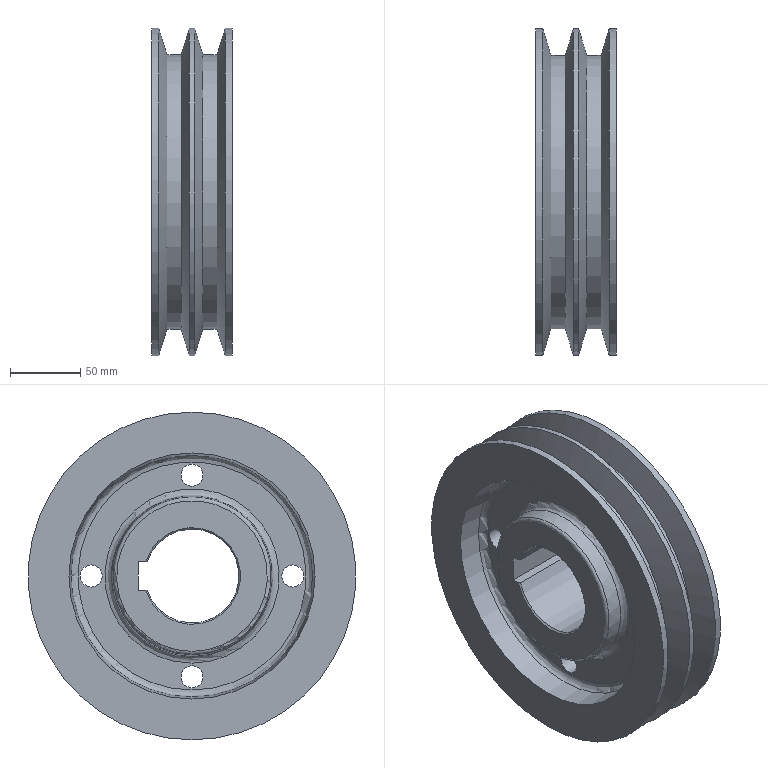Part | NX | features 大带轮_孔板轮(A) 2 | 1 solid | 35 faces | box 57.5 x 233.6 x 233.6 mm | volume 1208197 mm3 | cylinder 10 | cone 10 | plane 9 | torus 6 | commonest cylinder face diameters 15.7 x4 233.6 x3 195.4 x2 67 x1
STEP:
#1=CARTESIAN_POINT('',(21.25,0.,-62.113));
#2=VERTEX_POINT('',#1);
#3=CARTESIAN_POINT('',(21.25,0.,0.));
#4=DIRECTION('',(1.,0.,0.));
#5=DIRECTION('',(0.,0.,-1.));
#6=AXIS2_PLACEMENT_3D('',#3,#4,#5);
#7=CIRCLE('',#6,62.113);
#8=EDGE_CURVE('',#2,#2,#7,.T.);
#9=ORIENTED_EDGE('',*,*,#8,.T.);
#10=EDGE_LOOP('',(#9));
#11=FACE_BOUND('',#10,.T.);
#12=CARTESIAN_POINT('',(21.25,0.,-81.259));
#13=VERTEX_POINT('',#12);
#14=CARTESIAN_POINT('',(21.25,0.,0.));
#15=DIRECTION('',(1.,0.,0.));
#16=DIRECTION('',(0.,0.,-1.));
#17=AXIS2_PLACEMENT_3D('',#14,#15,#16);
#18=CIRCLE('',#17,81.259);
#19=EDGE_CURVE('',#13,#13,#18,.F.);
#20=ORIENTED_EDGE('',*,*,#19,.T.);
#21=EDGE_LOOP('',(#20));
#22=FACE_BOUND('',#21,.T.);
#23=CARTESIAN_POINT('',(21.25,71.85,-7.85));
#24=VERTEX_POINT('',#23);
#25=CARTESIAN_POINT('',(21.25,71.85,0.));
#26=DIRECTION('',(1.,0.,0.));
#27=DIRECTION('',(0.,0.,-1.));
#28=AXIS2_PLACEMENT_3D('',#25,#26,#27);
#29=CIRCLE('',#28,7.85);
#30=EDGE_CURVE('',#24,#24,#29,.F.);
#31=ORIENTED_EDGE('',*,*,#30,.F.);
#32=EDGE_LOOP('',(#31));
#33=FACE_BOUND('',#32,.T.);
#34=CARTESIAN_POINT('',(21.25,0.,-79.7));
#35=VERTEX_POINT('',#34);
#36=CARTESIAN_POINT('',(21.25,0.,-71.85));
#37=DIRECTION('',(1.,0.,0.));
#38=DIRECTION('',(0.,0.,-1.));
#39=AXIS2_PLACEMENT_3D('',#36,#37,#38);
#40=CIRCLE('',#39,7.85);
#41=EDGE_CURVE('',#35,#35,#40,.F.);
#42=ORIENTED_EDGE('',*,*,#41,.F.);
#43=EDGE_LOOP('',(#42));
#44=FACE_BOUND('',#43,.T.);
#45=CARTESIAN_POINT('',(21.25,-71.85,-7.85));
#46=VERTEX_POINT('',#45);
#47=CARTESIAN_POINT('',(21.25,-71.85,0.));
#48=DIRECTION('',(1.,0.,0.));
#49=DIRECTION('',(0.,0.,-1.));
#50=AXIS2_PLACEMENT_3D('',#47,#48,#49);
#51=CIRCLE('',#50,7.85);
#52=EDGE_CURVE('',#46,#46,#51,.F.);
#53=ORIENTED_EDGE('',*,*,#52,.F.);
#54=EDGE_LOOP('',(#53));
#55=FACE_BOUND('',#54,.T.);
#56=CARTESIAN_POINT('',(21.25,0.,64.));
#57=VERTEX_POINT('',#56);
#58=CARTESIAN_POINT('',(21.25,0.,71.85));
#59=DIRECTION('',(1.,0.,0.));
#60=DIRECTION('',(0.,0.,-1.));
#61=AXIS2_PLACEMENT_3D('',#58,#59,#60);
#62=CIRCLE('',#61,7.85);
#63=EDGE_CURVE('',#57,#57,#62,.F.);
#64=ORIENTED_EDGE('',*,*,#63,.F.);
#65=EDGE_LOOP('',(#64));
#66=FACE_BOUND('',#65,.T.);
#67=CARTESIAN_POINT('',(21.25,57.531,0.));
#68=DIRECTION('',(1.,0.,0.));
#69=DIRECTION('',(0.,0.,-1.));
#70=AXIS2_PLACEMENT_3D('',#67,#68,#69);
#71=PLANE('',#70);
#72=ADVANCED_FACE('',(#11,#22,#33,#44,#55,#66),#71,.F.);
#73=CARTESIAN_POINT('',(36.25,0.,62.113));
#74=VERTEX_POINT('',#73);
#75=CARTESIAN_POINT('',(36.25,0.,0.));
#76=DIRECTION('',(-1.,0.,0.));
#77=DIRECTION('',(0.,0.,1.));
#78=AXIS2_PLACEMENT_3D('',#75,#76,#77);
#79=CIRCLE('',#78,62.113);
#80=EDGE_CURVE('',#74,#74,#79,.T.);
#81=ORIENTED_EDGE('',*,*,#80,.T.);
#82=EDGE_LOOP('',(#81));
#83=FACE_BOUND('',#82,.T.);
#84=CARTESIAN_POINT('',(36.25,0.,81.259));
#85=VERTEX_POINT('',#84);
#86=CARTESIAN_POINT('',(36.25,0.,0.));
#87=DIRECTION('',(-1.,0.,0.));
#88=DIRECTION('',(0.,0.,1.));
#89=AXIS2_PLACEMENT_3D('',#86,#87,#88);
#90=CIRCLE('',#89,81.259);
#91=EDGE_CURVE('',#85,#85,#90,.F.);
#92=ORIENTED_EDGE('',*,*,#91,.T.);
#93=EDGE_LOOP('',(#92));
#94=FACE_BOUND('',#93,.T.);
#95=CARTESIAN_POINT('',(36.25,71.85,7.85));
#96=VERTEX_POINT('',#95);
#97=CARTESIAN_POINT('',(36.25,71.85,0.));
#98=DIRECTION('',(-1.,0.,0.));
#99=DIRECTION('',(0.,0.,1.));
#100=AXIS2_PLACEMENT_3D('',#97,#98,#99);
#101=CIRCLE('',#100,7.85);
#102=EDGE_CURVE('',#96,#96,#101,.F.);
#103=ORIENTED_EDGE('',*,*,#102,.F.);
#104=EDGE_LOOP('',(#103));
#105=FACE_BOUND('',#104,.T.);
#106=CARTESIAN_POINT('',(36.25,0.,-64.));
#107=VERTEX_POINT('',#106);
#108=CARTESIAN_POINT('',(36.25,0.,-71.85));
#109=DIRECTION('',(-1.,0.,0.));
#110=DIRECTION('',(0.,0.,1.));
#111=AXIS2_PLACEMENT_3D('',#108,#109,#110);
#112=CIRCLE('',#111,7.85);
#113=EDGE_CURVE('',#107,#107,#112,.F.);
#114=ORIENTED_EDGE('',*,*,#113,.F.);
#115=EDGE_LOOP('',(#114));
#116=FACE_BOUND('',#115,.T.);
#117=CARTESIAN_POINT('',(36.25,-71.85,7.85));
#118=VERTEX_POINT('',#117);
#119=CARTESIAN_POINT('',(36.25,-71.85,0.));
#120=DIRECTION('',(-1.,0.,0.));
#121=DIRECTION('',(0.,0.,1.));
#122=AXIS2_PLACEMENT_3D('',#119,#120,#121);
#123=CIRCLE('',#122,7.85);
#124=EDGE_CURVE('',#118,#118,#123,.F.);
#125=ORIENTED_EDGE('',*,*,#124,.F.);
#126=EDGE_LOOP('',(#125));
#127=FACE_BOUND('',#126,.T.);
#128=CARTESIAN_POINT('',(36.25,0.,79.7));
#129=VERTEX_POINT('',#128);
#130=CARTESIAN_POINT('',(36.25,0.,71.85));
#131=DIRECTION('',(-1.,0.,0.));
#132=DIRECTION('',(0.,0.,1.));
#133=AXIS2_PLACEMENT_3D('',#130,#131,#132);
#134=CIRCLE('',#133,7.85);
#135=EDGE_CURVE('',#129,#129,#134,.F.);
#136=ORIENTED_EDGE('',*,*,#135,.F.);
#137=EDGE_LOOP('',(#136));
#138=FACE_BOUND('',#137,.T.);
#139=CARTESIAN_POINT('',(36.25,85.841,0.));
#140=DIRECTION('',(-1.,0.,0.));
#141=DIRECTION('',(0.,0.,1.));
#142=AXIS2_PLACEMENT_3D('',#139,#140,#141);
#143=PLANE('',#142);
#144=ADVANCED_FACE('',(#83,#94,#105,#116,#127,#138),#143,.F.);
#145=CARTESIAN_POINT('',(57.5,0.,116.8));
#146=VERTEX_POINT('',#145);
#147=CARTESIAN_POINT('',(57.5,0.,0.));
#148=DIRECTION('',(-1.,0.,0.));
#149=DIRECTION('',(0.,0.,1.));
#150=AXIS2_PLACEMENT_3D('',#147,#148,#149);
#151=CIRCLE('',#150,116.8);
#152=EDGE_CURVE('',#146,#146,#151,.T.);
#153=ORIENTED_EDGE('',*,*,#152,.T.);
#154=EDGE_LOOP('',(#153));
#155=FACE_BOUND('',#154,.T.);
#156=CARTESIAN_POINT('',(52.468,0.,116.8));
#157=VERTEX_POINT('',#156);
#158=CARTESIAN_POINT('',(52.468,0.,0.));
#159=DIRECTION('',(-1.,0.,0.));
#160=DIRECTION('',(0.,0.,1.));
#161=AXIS2_PLACEMENT_3D('',#158,#159,#160);
#162=CIRCLE('',#161,116.8);
#163=EDGE_CURVE('',#157,#157,#162,.T.);
#164=ORIENTED_EDGE('',*,*,#163,.F.);
#165=EDGE_LOOP('',(#164));
#166=FACE_BOUND('',#165,.T.);
#167=CARTESIAN_POINT('',(0.,0.,0.));
#168=DIRECTION('',(-1.,0.,0.));
#169=DIRECTION('',(0.,0.,1.));
#170=AXIS2_PLACEMENT_3D('',#167,#168,#169);
#171=CYLINDRICAL_SURFACE('',#170,116.8);
#172=ADVANCED_FACE('',(#155,#166),#171,.T.);
#173=CARTESIAN_POINT('',(26.968,0.,116.8));
#174=VERTEX_POINT('',#173);
#175=CARTESIAN_POINT('',(26.968,0.,0.));
#176=DIRECTION('',(-1.,0.,0.));
#177=DIRECTION('',(0.,0.,1.));
#178=AXIS2_PLACEMENT_3D('',#175,#176,#177);
#179=CIRCLE('',#178,116.8);
#180=EDGE_CURVE('',#174,#174,#179,.T.);
#181=ORIENTED_EDGE('',*,*,#180,.F.);
#182=EDGE_LOOP('',(#181));
#183=FACE_BOUND('',#182,.T.);
#184=CARTESIAN_POINT('',(30.532,0.,116.8));
#185=VERTEX_POINT('',#184);
#186=CARTESIAN_POINT('',(30.532,0.,0.));
#187=DIRECTION('',(-1.,0.,0.));
#188=DIRECTION('',(0.,0.,1.));
#189=AXIS2_PLACEMENT_3D('',#186,#187,#188);
#190=CIRCLE('',#189,116.8);
#191=EDGE_CURVE('',#185,#185,#190,.T.);
#192=ORIENTED_EDGE('',*,*,#191,.T.);
#193=EDGE_LOOP('',(#192));
#194=FACE_BOUND('',#193,.T.);
#195=CARTESIAN_POINT('',(0.,0.,0.));
#196=DIRECTION('',(-1.,0.,0.));
#197=DIRECTION('',(0.,0.,1.));
#198=AXIS2_PLACEMENT_3D('',#195,#196,#197);
#199=CYLINDRICAL_SURFACE('',#198,116.8);
#200=ADVANCED_FACE('',(#183,#194),#199,.T.);
#201=CARTESIAN_POINT('',(0.,0.,116.8));
#202=VERTEX_POINT('',#201);
#203=CARTESIAN_POINT('',(0.,0.,0.));
#204=DIRECTION('',(-1.,0.,0.));
#205=DIRECTION('',(0.,0.,1.));
#206=AXIS2_PLACEMENT_3D('',#203,#204,#205);
#207=CIRCLE('',#206,116.8);
#208=EDGE_CURVE('',#202,#202,#207,.T.);
#209=ORIENTED_EDGE('',*,*,#208,.F.);
#210=EDGE_LOOP('',(#209));
#211=FACE_BOUND('',#210,.T.);
#212=CARTESIAN_POINT('',(5.032,0.,116.8));
#213=VERTEX_POINT('',#212);
#214=CARTESIAN_POINT('',(5.032,0.,0.));
#215=DIRECTION('',(-1.,0.,0.));
#216=DIRECTION('',(0.,0.,1.));
#217=AXIS2_PLACEMENT_3D('',#214,#215,#216);
#218=CIRCLE('',#217,116.8);
#219=EDGE_CURVE('',#213,#213,#218,.T.);
#220=ORIENTED_EDGE('',*,*,#219,.T.);
#221=EDGE_LOOP('',(#220));
#222=FACE_BOUND('',#221,.T.);
#223=CARTESIAN_POINT('',(0.,0.,0.));
#224=DIRECTION('',(-1.,0.,0.));
#225=DIRECTION('',(0.,0.,1.));
#226=AXIS2_PLACEMENT_3D('',#223,#224,#225);
#227=CYLINDRICAL_SURFACE('',#226,116.8);
#228=ADVANCED_FACE('',(#211,#222),#227,.T.);
#229=CARTESIAN_POINT('',(4.75,31.973,-10.));
#230=VERTEX_POINT('',#229);
#231=CARTESIAN_POINT('',(4.75,31.973,10.));
#232=VERTEX_POINT('',#231);
#233=CARTESIAN_POINT('',(4.75,0.,0.));
#234=DIRECTION('',(1.,0.,0.));
#235=DIRECTION('',(0.,0.,-1.));
#236=AXIS2_PLACEMENT_3D('',#233,#234,#235);
#237=CIRCLE('',#236,33.5);
#238=EDGE_CURVE('',#230,#232,#237,.F.);
#239=ORIENTED_EDGE('',*,*,#238,.T.);
#240=CARTESIAN_POINT('',(52.75,31.973,10.));
#241=VERTEX_POINT('',#240);
#242=CARTESIAN_POINT('',(57.5,31.973,10.));
#243=DIRECTION('',(-1.,0.,0.));
#244=VECTOR('',#243,1000.);
#245=LINE('',#242,#244);
#246=EDGE_CURVE('',#241,#232,#245,.T.);
#247=ORIENTED_EDGE('',*,*,#246,.F.);
#248=CARTESIAN_POINT('',(52.75,31.973,-10.));
#249=VERTEX_POINT('',#248);
#250=CARTESIAN_POINT('',(52.75,0.,0.));
#251=DIRECTION('',(-1.,0.,0.));
#252=DIRECTION('',(0.,0.,1.));
#253=AXIS2_PLACEMENT_3D('',#250,#251,#252);
#254=CIRCLE('',#253,33.5);
#255=EDGE_CURVE('',#241,#249,#254,.F.);
#256=ORIENTED_EDGE('',*,*,#255,.T.);
#257=CARTESIAN_POINT('',(57.5,31.973,-10.));
#258=DIRECTION('',(-1.,0.,0.));
#259=VECTOR('',#258,1000.);
#260=LINE('',#257,#259);
#261=EDGE_CURVE('',#249,#230,#260,.T.);
#262=ORIENTED_EDGE('',*,*,#261,.T.);
#263=EDGE_LOOP('',(#239,#247,#256,#262));
#264=FACE_BOUND('',#263,.T.);
#265=CARTESIAN_POINT('',(0.,0.,0.));
#266=DIRECTION('',(-1.,0.,0.));
#267=DIRECTION('',(0.,0.,1.));
#268=AXIS2_PLACEMENT_3D('',#265,#266,#267);
#269=CYLINDRICAL_SURFACE('',#268,33.5);
#270=ADVANCED_FACE('',(#264),#269,.F.);
#271=CARTESIAN_POINT('',(3.75,0.,-53.709));
#272=VERTEX_POINT('',#271);
#273=CARTESIAN_POINT('',(3.75,0.,0.));
#274=DIRECTION('',(1.,0.,0.));
#275=DIRECTION('',(0.,0.,-1.));
#276=AXIS2_PLACEMENT_3D('',#273,#274,#275);
#277=CIRCLE('',#276,53.709);
#278=EDGE_CURVE('',#272,#272,#277,.F.);
#279=ORIENTED_EDGE('',*,*,#278,.T.);
#280=EDGE_LOOP('',(#279));
#281=FACE_BOUND('',#280,.T.);
#282=CARTESIAN_POINT('',(3.75,33.019,10.));
#283=VERTEX_POINT('',#282);
#284=CARTESIAN_POINT('',(3.75,33.019,-10.));
#285=VERTEX_POINT('',#284);
#286=CARTESIAN_POINT('',(3.75,0.,0.));
#287=DIRECTION('',(1.,0.,0.));
#288=DIRECTION('',(0.,0.,-1.));
#289=AXIS2_PLACEMENT_3D('',#286,#287,#288);
#290=CIRCLE('',#289,34.5);
#291=EDGE_CURVE('',#283,#285,#290,.T.);
#292=ORIENTED_EDGE('',*,*,#291,.T.);
#293=CARTESIAN_POINT('',(3.75,38.4,-10.));
#294=VERTEX_POINT('',#293);
#295=CARTESIAN_POINT('',(3.75,31.973,-10.));
#296=DIRECTION('',(0.,-1.,0.));
#297=VECTOR('',#296,1000.);
#298=LINE('',#295,#297);
#299=EDGE_CURVE('',#294,#285,#298,.T.);
#300=ORIENTED_EDGE('',*,*,#299,.F.);
#301=CARTESIAN_POINT('',(3.75,38.4,10.));
#302=VERTEX_POINT('',#301);
#303=CARTESIAN_POINT('',(3.75,38.4,-10.));
#304=DIRECTION('',(0.,0.,-1.));
#305=VECTOR('',#304,1000.);
#306=LINE('',#303,#305);
#307=EDGE_CURVE('',#302,#294,#306,.T.);
#308=ORIENTED_EDGE('',*,*,#307,.F.);
#309=CARTESIAN_POINT('',(3.75,31.973,10.));
#310=DIRECTION('',(0.,1.,0.));
#311=VECTOR('',#310,1000.);
#312=LINE('',#309,#311);
#313=EDGE_CURVE('',#283,#302,#312,.T.);
#314=ORIENTED_EDGE('',*,*,#313,.F.);
#315=EDGE_LOOP('',(#292,#300,#308,#314));
#316=FACE_BOUND('',#315,.T.);
#317=CARTESIAN_POINT('',(3.75,33.5,0.));
#318=DIRECTION('',(1.,0.,0.));
#319=DIRECTION('',(0.,0.,-1.));
#320=AXIS2_PLACEMENT_3D('',#317,#318,#319);
#321=PLANE('',#320);
#322=ADVANCED_FACE('',(#281,#316),#321,.F.);
#323=CARTESIAN_POINT('',(6.032,0.,56.2));
#324=VERTEX_POINT('',#323);
#325=CARTESIAN_POINT('',(6.032,0.,0.));
#326=DIRECTION('',(-1.,0.,0.));
#327=DIRECTION('',(0.,0.,1.));
#328=AXIS2_PLACEMENT_3D('',#325,#326,#327);
#329=CIRCLE('',#328,56.2);
#330=EDGE_CURVE('',#324,#324,#329,.F.);
#331=ORIENTED_EDGE('',*,*,#330,.T.);
#332=EDGE_LOOP('',(#331));
#333=FACE_BOUND('',#332,.T.);
#334=CARTESIAN_POINT('',(16.686,0.,-57.132));
#335=VERTEX_POINT('',#334);
#336=CARTESIAN_POINT('',(16.686,0.,0.));
#337=DIRECTION('',(1.,0.,0.));
#338=DIRECTION('',(0.,0.,-1.));
#339=AXIS2_PLACEMENT_3D('',#336,#337,#338);
#340=CIRCLE('',#339,57.132);
#341=EDGE_CURVE('',#335,#335,#340,.F.);
#342=ORIENTED_EDGE('',*,*,#341,.T.);
#343=EDGE_LOOP('',(#342));
#344=FACE_BOUND('',#343,.T.);
#345=CARTESIAN_POINT('',(21.25,0.,0.));
#346=DIRECTION('',(1.,0.,0.));
#347=DIRECTION('',(0.,0.,-1.));
#348=AXIS2_PLACEMENT_3D('',#345,#346,#347);
#349=CONICAL_SURFACE('',#348,57.531,0.08727);
#350=ADVANCED_FACE('',(#333,#344),#349,.T.);
#351=CARTESIAN_POINT('',(16.686,0.,86.24));
#352=VERTEX_POINT('',#351);
#353=CARTESIAN_POINT('',(16.686,0.,0.));
#354=DIRECTION('',(-1.,0.,0.));
#355=DIRECTION('',(0.,0.,1.));
#356=AXIS2_PLACEMENT_3D('',#353,#354,#355);
#357=CIRCLE('',#356,86.24);
#358=EDGE_CURVE('',#352,#352,#357,.F.);
#359=ORIENTED_EDGE('',*,*,#358,.T.);
#360=EDGE_LOOP('',(#359));
#361=FACE_BOUND('',#360,.T.);
#362=CARTESIAN_POINT('',(0.,0.,87.7));
#363=VERTEX_POINT('',#362);
#364=CARTESIAN_POINT('',(0.,0.,0.));
#365=DIRECTION('',(-1.,0.,0.));
#366=DIRECTION('',(0.,0.,1.));
#367=AXIS2_PLACEMENT_3D('',#364,#365,#366);
#368=CIRCLE('',#367,87.7);
#369=EDGE_CURVE('',#363,#363,#368,.T.);
#370=ORIENTED_EDGE('',*,*,#369,.T.);
#371=EDGE_LOOP('',(#370));
#372=FACE_BOUND('',#371,.T.);
#373=CARTESIAN_POINT('',(0.,0.,0.));
#374=DIRECTION('',(-1.,0.,0.));
#375=DIRECTION('',(0.,0.,1.));
#376=AXIS2_PLACEMENT_3D('',#373,#374,#375);
#377=CONICAL_SURFACE('',#376,87.7,0.08727);
#378=ADVANCED_FACE('',(#361,#372),#377,.F.);
#379=ORIENTED_EDGE('',*,*,#369,.F.);
#380=EDGE_LOOP('',(#379));
#381=FACE_BOUND('',#380,.T.);
#382=ORIENTED_EDGE('',*,*,#208,.T.);
#383=EDGE_LOOP('',(#382));
#384=FACE_BOUND('',#383,.T.);
#385=CARTESIAN_POINT('',(0.,87.7,0.));
#386=DIRECTION('',(1.,0.,0.));
#387=DIRECTION('',(0.,0.,-1.));
#388=AXIS2_PLACEMENT_3D('',#385,#386,#387);
#389=PLANE('',#388);
#390=ADVANCED_FACE('',(#381,#384),#389,.F.);
#391=ORIENTED_EDGE('',*,*,#152,.F.);
#392=EDGE_LOOP('',(#391));
#393=FACE_BOUND('',#392,.T.);
#394=CARTESIAN_POINT('',(57.5,0.,87.7));
#395=VERTEX_POINT('',#394);
#396=CARTESIAN_POINT('',(57.5,0.,0.));
#397=DIRECTION('',(-1.,0.,0.));
#398=DIRECTION('',(0.,0.,1.));
#399=AXIS2_PLACEMENT_3D('',#396,#397,#398);
#400=CIRCLE('',#399,87.7);
#401=EDGE_CURVE('',#395,#395,#400,.T.);
#402=ORIENTED_EDGE('',*,*,#401,.T.);
#403=EDGE_LOOP('',(#402));
#404=FACE_BOUND('',#403,.T.);
#405=CARTESIAN_POINT('',(57.5,116.8,0.));
#406=DIRECTION('',(-1.,0.,0.));
#407=DIRECTION('',(0.,0.,1.));
#408=AXIS2_PLACEMENT_3D('',#405,#406,#407);
#409=PLANE('',#408);
#410=ADVANCED_FACE('',(#393,#404),#409,.F.);
#411=CARTESIAN_POINT('',(40.814,0.,-86.24));
#412=VERTEX_POINT('',#411);
#413=CARTESIAN_POINT('',(40.814,0.,0.));
#414=DIRECTION('',(1.,0.,0.));
#415=DIRECTION('',(0.,0.,-1.));
#416=AXIS2_PLACEMENT_3D('',#413,#414,#415);
#417=CIRCLE('',#416,86.24);
#418=EDGE_CURVE('',#412,#412,#417,.F.);
#419=ORIENTED_EDGE('',*,*,#418,.T.);
#420=EDGE_LOOP('',(#419));
#421=FACE_BOUND('',#420,.T.);
#422=ORIENTED_EDGE('',*,*,#401,.F.);
#423=EDGE_LOOP('',(#422));
#424=FACE_BOUND('',#423,.T.);
#425=CARTESIAN_POINT('',(36.25,0.,0.));
#426=DIRECTION('',(1.,0.,0.));
#427=DIRECTION('',(0.,0.,-1.));
#428=AXIS2_PLACEMENT_3D('',#425,#426,#427);
#429=CONICAL_SURFACE('',#428,85.841,0.08727);
#430=ADVANCED_FACE('',(#421,#424),#429,.F.);
#431=CARTESIAN_POINT('',(51.468,0.,-56.2));
#432=VERTEX_POINT('',#431);
#433=CARTESIAN_POINT('',(51.468,0.,0.));
#434=DIRECTION('',(1.,0.,0.));
#435=DIRECTION('',(0.,0.,-1.));
#436=AXIS2_PLACEMENT_3D('',#433,#434,#435);
#437=CIRCLE('',#436,56.2);
#438=EDGE_CURVE('',#432,#432,#437,.F.);
#439=ORIENTED_EDGE('',*,*,#438,.T.);
#440=EDGE_LOOP('',(#439));
#441=FACE_BOUND('',#440,.T.);
#442=CARTESIAN_POINT('',(40.814,0.,57.132));
#443=VERTEX_POINT('',#442);
#444=CARTESIAN_POINT('',(40.814,0.,0.));
#445=DIRECTION('',(-1.,0.,0.));
#446=DIRECTION('',(0.,0.,1.));
#447=AXIS2_PLACEMENT_3D('',#444,#445,#446);
#448=CIRCLE('',#447,57.132);
#449=EDGE_CURVE('',#443,#443,#448,.F.);
#450=ORIENTED_EDGE('',*,*,#449,.T.);
#451=EDGE_LOOP('',(#450));
#452=FACE_BOUND('',#451,.T.);
#453=CARTESIAN_POINT('',(53.75,0.,0.));
#454=DIRECTION('',(-1.,0.,0.));
#455=DIRECTION('',(0.,0.,1.));
#456=AXIS2_PLACEMENT_3D('',#453,#454,#455);
#457=CONICAL_SURFACE('',#456,56.,0.08727);
#458=ADVANCED_FACE('',(#441,#452),#457,.T.);
#459=CARTESIAN_POINT('',(53.75,0.,53.709));
#460=VERTEX_POINT('',#459);
#461=CARTESIAN_POINT('',(53.75,0.,0.));
#462=DIRECTION('',(-1.,0.,0.));
#463=DIRECTION('',(0.,0.,1.));
#464=AXIS2_PLACEMENT_3D('',#461,#462,#463);
#465=CIRCLE('',#464,53.709);
#466=EDGE_CURVE('',#460,#460,#465,.F.);
#467=ORIENTED_EDGE('',*,*,#466,.T.);
#468=EDGE_LOOP('',(#467));
#469=FACE_BOUND('',#468,.T.);
#470=CARTESIAN_POINT('',(53.75,38.4,10.));
#471=VERTEX_POINT('',#470);
#472=CARTESIAN_POINT('',(53.75,38.4,-10.));
#473=VERTEX_POINT('',#472);
#474=CARTESIAN_POINT('',(53.75,38.4,0.));
#475=DIRECTION('',(0.,0.,-1.));
#476=VECTOR('',#475,1000.);
#477=LINE('',#474,#476);
#478=EDGE_CURVE('',#471,#473,#477,.T.);
#479=ORIENTED_EDGE('',*,*,#478,.T.);
#480=CARTESIAN_POINT('',(53.75,33.019,-10.));
#481=VERTEX_POINT('',#480);
#482=CARTESIAN_POINT('',(53.75,56.,-10.));
#483=DIRECTION('',(0.,-1.,0.));
#484=VECTOR('',#483,1000.);
#485=LINE('',#482,#484);
#486=EDGE_CURVE('',#473,#481,#485,.T.);
#487=ORIENTED_EDGE('',*,*,#486,.T.);
#488=CARTESIAN_POINT('',(53.75,33.019,10.));
#489=VERTEX_POINT('',#488);
#490=CARTESIAN_POINT('',(53.75,0.,0.));
#491=DIRECTION('',(-1.,0.,0.));
#492=DIRECTION('',(0.,0.,1.));
#493=AXIS2_PLACEMENT_3D('',#490,#491,#492);
#494=CIRCLE('',#493,34.5);
#495=EDGE_CURVE('',#481,#489,#494,.T.);
#496=ORIENTED_EDGE('',*,*,#495,.T.);
#497=CARTESIAN_POINT('',(53.75,56.,10.));
#498=DIRECTION('',(0.,1.,0.));
#499=VECTOR('',#498,1000.);
#500=LINE('',#497,#499);
#501=EDGE_CURVE('',#489,#471,#500,.T.);
#502=ORIENTED_EDGE('',*,*,#501,.T.);
#503=EDGE_LOOP('',(#479,#487,#496,#502));
#504=FACE_BOUND('',#503,.T.);
#505=CARTESIAN_POINT('',(53.75,56.,0.));
#506=DIRECTION('',(-1.,0.,0.));
#507=DIRECTION('',(0.,0.,1.));
#508=AXIS2_PLACEMENT_3D('',#505,#506,#507);
#509=PLANE('',#508);
#510=ADVANCED_FACE('',(#469,#504),#509,.F.);
#511=CARTESIAN_POINT('',(21.128,0.,97.7));
#512=VERTEX_POINT('',#511);
#513=CARTESIAN_POINT('',(21.128,0.,0.));
#514=DIRECTION('',(-1.,0.,0.));
#515=DIRECTION('',(0.,0.,1.));
#516=AXIS2_PLACEMENT_3D('',#513,#514,#515);
#517=CIRCLE('',#516,97.7);
#518=EDGE_CURVE('',#512,#512,#517,.T.);
#519=ORIENTED_EDGE('',*,*,#518,.T.);
#520=EDGE_LOOP('',(#519));
#521=FACE_BOUND('',#520,.T.);
#522=CARTESIAN_POINT('',(10.872,0.,97.7));
#523=VERTEX_POINT('',#522);
#524=CARTESIAN_POINT('',(10.872,0.,0.));
#525=DIRECTION('',(-1.,0.,0.));
#526=DIRECTION('',(0.,0.,1.));
#527=AXIS2_PLACEMENT_3D('',#524,#525,#526);
#528=CIRCLE('',#527,97.7);
#529=EDGE_CURVE('',#523,#523,#528,.T.);
#530=ORIENTED_EDGE('',*,*,#529,.F.);
#531=EDGE_LOOP('',(#530));
#532=FACE_BOUND('',#531,.T.);
#533=CARTESIAN_POINT('',(0.,0.,0.));
#534=DIRECTION('',(-1.,0.,0.));
#535=DIRECTION('',(0.,0.,1.));
#536=AXIS2_PLACEMENT_3D('',#533,#534,#535);
#537=CYLINDRICAL_SURFACE('',#536,97.7);
#538=ADVANCED_FACE('',(#521,#532),#537,.T.);
#539=ORIENTED_EDGE('',*,*,#180,.T.);
#540=EDGE_LOOP('',(#539));
#541=FACE_BOUND('',#540,.T.);
#542=ORIENTED_EDGE('',*,*,#518,.F.);
#543=EDGE_LOOP('',(#542));
#544=FACE_BOUND('',#543,.T.);
#545=CARTESIAN_POINT('',(21.128,0.,0.));
#546=DIRECTION('',(1.,0.,0.));
#547=DIRECTION('',(0.,0.,-1.));
#548=AXIS2_PLACEMENT_3D('',#545,#546,#547);
#549=CONICAL_SURFACE('',#548,97.7,1.274);
#550=ADVANCED_FACE('',(#541,#544),#549,.T.);
#551=ORIENTED_EDGE('',*,*,#529,.T.);
#552=EDGE_LOOP('',(#551));
#553=FACE_BOUND('',#552,.T.);
#554=ORIENTED_EDGE('',*,*,#219,.F.);
#555=EDGE_LOOP('',(#554));
#556=FACE_BOUND('',#555,.T.);
#557=CARTESIAN_POINT('',(5.032,0.,0.));
#558=DIRECTION('',(-1.,0.,0.));
#559=DIRECTION('',(0.,0.,1.));
#560=AXIS2_PLACEMENT_3D('',#557,#558,#559);
#561=CONICAL_SURFACE('',#560,116.8,1.274);
#562=ADVANCED_FACE('',(#553,#556),#561,.T.);
#563=CARTESIAN_POINT('',(46.628,0.,97.7));
#564=VERTEX_POINT('',#563);
#565=CARTESIAN_POINT('',(46.628,0.,0.));
#566=DIRECTION('',(-1.,0.,0.));
#567=DIRECTION('',(0.,0.,1.));
#568=AXIS2_PLACEMENT_3D('',#565,#566,#567);
#569=CIRCLE('',#568,97.7);
#570=EDGE_CURVE('',#564,#564,#569,.T.);
#571=ORIENTED_EDGE('',*,*,#570,.T.);
#572=EDGE_LOOP('',(#571));
#573=FACE_BOUND('',#572,.T.);
#574=CARTESIAN_POINT('',(36.372,0.,97.7));
#575=VERTEX_POINT('',#574);
#576=CARTESIAN_POINT('',(36.372,0.,0.));
#577=DIRECTION('',(-1.,0.,0.));
#578=DIRECTION('',(0.,0.,1.));
#579=AXIS2_PLACEMENT_3D('',#576,#577,#578);
#580=CIRCLE('',#579,97.7);
#581=EDGE_CURVE('',#575,#575,#580,.T.);
#582=ORIENTED_EDGE('',*,*,#581,.F.);
#583=EDGE_LOOP('',(#582));
#584=FACE_BOUND('',#583,.T.);
#585=CARTESIAN_POINT('',(25.5,0.,0.));
#586=DIRECTION('',(-1.,0.,0.));
#587=DIRECTION('',(0.,0.,1.));
#588=AXIS2_PLACEMENT_3D('',#585,#586,#587);
#589=CYLINDRICAL_SURFACE('',#588,97.7);
#590=ADVANCED_FACE('',(#573,#584),#589,.T.);
#591=ORIENTED_EDGE('',*,*,#163,.T.);
#592=EDGE_LOOP('',(#591));
#593=FACE_BOUND('',#592,.T.);
#594=ORIENTED_EDGE('',*,*,#570,.F.);
#595=EDGE_LOOP('',(#594));
#596=FACE_BOUND('',#595,.T.);
#597=CARTESIAN_POINT('',(46.628,0.,0.));
#598=DIRECTION('',(1.,0.,0.));
#599=DIRECTION('',(0.,0.,-1.));
#600=AXIS2_PLACEMENT_3D('',#597,#598,#599);
#601=CONICAL_SURFACE('',#600,97.7,1.274);
#602=ADVANCED_FACE('',(#593,#596),#601,.T.);
#603=ORIENTED_EDGE('',*,*,#581,.T.);
#604=EDGE_LOOP('',(#603));
#605=FACE_BOUND('',#604,.T.);
#606=ORIENTED_EDGE('',*,*,#191,.F.);
#607=EDGE_LOOP('',(#606));
#608=FACE_BOUND('',#607,.T.);
#609=CARTESIAN_POINT('',(30.532,0.,0.));
#610=DIRECTION('',(-1.,0.,0.));
#611=DIRECTION('',(0.,0.,1.));
#612=AXIS2_PLACEMENT_3D('',#609,#610,#611);
#613=CONICAL_SURFACE('',#612,116.8,1.274);
#614=ADVANCED_FACE('',(#605,#608),#613,.T.);
#615=CARTESIAN_POINT('',(3.75,33.019,-10.));
#616=CARTESIAN_POINT('',(4.084,32.67,-10.));
#617=CARTESIAN_POINT('',(4.417,32.322,-10.));
#618=CARTESIAN_POINT('',(4.75,31.973,-10.));
#619=B_SPLINE_CURVE_WITH_KNOTS('',3,(#615,#616,#617,#618),.UNSPECIFIED.,.F.,.F.,(4,4),(0.004576,0.006023),.UNSPECIFIED.);
#620=EDGE_CURVE('',#285,#230,#619,.T.);
#621=ORIENTED_EDGE('',*,*,#620,.F.);
#622=ORIENTED_EDGE('',*,*,#291,.F.);
#623=CARTESIAN_POINT('',(4.75,31.973,10.));
#624=CARTESIAN_POINT('',(4.417,32.322,10.));
#625=CARTESIAN_POINT('',(4.084,32.67,10.));
#626=CARTESIAN_POINT('',(3.75,33.019,10.));
#627=B_SPLINE_CURVE_WITH_KNOTS('',3,(#623,#624,#625,#626),.UNSPECIFIED.,.F.,.F.,(4,4),(0.004876,0.006323),.UNSPECIFIED.);
#628=EDGE_CURVE('',#232,#283,#627,.T.);
#629=ORIENTED_EDGE('',*,*,#628,.F.);
#630=ORIENTED_EDGE('',*,*,#238,.F.);
#631=EDGE_LOOP('',(#621,#622,#629,#630));
#632=FACE_BOUND('',#631,.T.);
#633=CARTESIAN_POINT('',(4.75,0.,0.));
#634=DIRECTION('',(-1.,0.,0.));
#635=DIRECTION('',(0.,0.,1.));
#636=AXIS2_PLACEMENT_3D('',#633,#634,#635);
#637=CONICAL_SURFACE('',#636,33.5,0.7854);
#638=ADVANCED_FACE('',(#632),#637,.F.);
#639=CARTESIAN_POINT('',(52.75,31.973,-10.));
#640=CARTESIAN_POINT('',(53.083,32.322,-10.));
#641=CARTESIAN_POINT('',(53.416,32.67,-10.));
#642=CARTESIAN_POINT('',(53.75,33.019,-10.));
#643=B_SPLINE_CURVE_WITH_KNOTS('',3,(#639,#640,#641,#642),.UNSPECIFIED.,.F.,.F.,(4,4),(0.004876,0.006323),.UNSPECIFIED.);
#644=EDGE_CURVE('',#249,#481,#643,.T.);
#645=ORIENTED_EDGE('',*,*,#644,.F.);
#646=ORIENTED_EDGE('',*,*,#255,.F.);
#647=CARTESIAN_POINT('',(53.75,33.019,10.));
#648=CARTESIAN_POINT('',(53.416,32.67,10.));
#649=CARTESIAN_POINT('',(53.083,32.322,10.));
#650=CARTESIAN_POINT('',(52.75,31.973,10.));
#651=B_SPLINE_CURVE_WITH_KNOTS('',3,(#647,#648,#649,#650),.UNSPECIFIED.,.F.,.F.,(4,4),(0.004576,0.006023),.UNSPECIFIED.);
#652=EDGE_CURVE('',#489,#241,#651,.T.);
#653=ORIENTED_EDGE('',*,*,#652,.F.);
#654=ORIENTED_EDGE('',*,*,#495,.F.);
#655=EDGE_LOOP('',(#645,#646,#653,#654));
#656=FACE_BOUND('',#655,.T.);
#657=CARTESIAN_POINT('',(53.75,0.,0.));
#658=DIRECTION('',(1.,0.,0.));
#659=DIRECTION('',(0.,0.,-1.));
#660=AXIS2_PLACEMENT_3D('',#657,#658,#659);
#661=CONICAL_SURFACE('',#660,34.5,0.7854);
#662=ADVANCED_FACE('',(#656),#661,.F.);
#663=CARTESIAN_POINT('',(57.5,38.4,10.));
#664=DIRECTION('',(-1.,0.,0.));
#665=VECTOR('',#664,1000.);
#666=LINE('',#663,#665);
#667=EDGE_CURVE('',#471,#302,#666,.T.);
#668=ORIENTED_EDGE('',*,*,#667,.T.);
#669=ORIENTED_EDGE('',*,*,#307,.T.);
#670=CARTESIAN_POINT('',(57.5,38.4,-10.));
#671=DIRECTION('',(-1.,0.,0.));
#672=VECTOR('',#671,1000.);
#673=LINE('',#670,#672);
#674=EDGE_CURVE('',#473,#294,#673,.T.);
#675=ORIENTED_EDGE('',*,*,#674,.F.);
#676=ORIENTED_EDGE('',*,*,#478,.F.);
#677=EDGE_LOOP('',(#668,#669,#675,#676));
#678=FACE_BOUND('',#677,.T.);
#679=CARTESIAN_POINT('',(57.5,38.4,-10.));
#680=DIRECTION('',(0.,1.,0.));
#681=DIRECTION('',(0.,0.,1.));
#682=AXIS2_PLACEMENT_3D('',#679,#680,#681);
#683=PLANE('',#682);
#684=ADVANCED_FACE('',(#678),#683,.F.);
#685=ORIENTED_EDGE('',*,*,#620,.T.);
#686=ORIENTED_EDGE('',*,*,#261,.F.);
#687=ORIENTED_EDGE('',*,*,#644,.T.);
#688=ORIENTED_EDGE('',*,*,#486,.F.);
#689=ORIENTED_EDGE('',*,*,#674,.T.);
#690=ORIENTED_EDGE('',*,*,#299,.T.);
#691=EDGE_LOOP('',(#685,#686,#687,#688,#689,#690));
#692=FACE_BOUND('',#691,.T.);
#693=CARTESIAN_POINT('',(57.5,31.973,-10.));
#694=DIRECTION('',(0.,0.,-1.));
#695=DIRECTION('',(-1.,0.,0.));
#696=AXIS2_PLACEMENT_3D('',#693,#694,#695);
#697=PLANE('',#696);
#698=ADVANCED_FACE('',(#692),#697,.F.);
#699=ORIENTED_EDGE('',*,*,#628,.T.);
#700=ORIENTED_EDGE('',*,*,#313,.T.);
#701=ORIENTED_EDGE('',*,*,#667,.F.);
#702=ORIENTED_EDGE('',*,*,#501,.F.);
#703=ORIENTED_EDGE('',*,*,#652,.T.);
#704=ORIENTED_EDGE('',*,*,#246,.T.);
#705=EDGE_LOOP('',(#699,#700,#701,#702,#703,#704));
#706=FACE_BOUND('',#705,.T.);
#707=CARTESIAN_POINT('',(57.5,31.973,10.));
#708=DIRECTION('',(0.,0.,1.));
#709=DIRECTION('',(1.,0.,0.));
#710=AXIS2_PLACEMENT_3D('',#707,#708,#709);
#711=PLANE('',#710);
#712=ADVANCED_FACE('',(#706),#711,.F.);
#713=ORIENTED_EDGE('',*,*,#8,.F.);
#714=EDGE_LOOP('',(#713));
#715=FACE_BOUND('',#714,.T.);
#716=ORIENTED_EDGE('',*,*,#341,.F.);
#717=EDGE_LOOP('',(#716));
#718=FACE_BOUND('',#717,.T.);
#719=CARTESIAN_POINT('',(16.25,0.,0.));
#720=DIRECTION('',(1.,0.,0.));
#721=DIRECTION('',(0.,0.,-1.));
#722=AXIS2_PLACEMENT_3D('',#719,#720,#721);
#723=TOROIDAL_SURFACE('',#722,62.113,5.);
#724=ADVANCED_FACE('',(#715,#718),#723,.F.);
#725=ORIENTED_EDGE('',*,*,#358,.F.);
#726=EDGE_LOOP('',(#725));
#727=FACE_BOUND('',#726,.T.);
#728=ORIENTED_EDGE('',*,*,#19,.F.);
#729=EDGE_LOOP('',(#728));
#730=FACE_BOUND('',#729,.T.);
#731=CARTESIAN_POINT('',(16.25,0.,0.));
#732=DIRECTION('',(1.,0.,0.));
#733=DIRECTION('',(0.,0.,-1.));
#734=AXIS2_PLACEMENT_3D('',#731,#732,#733);
#735=TOROIDAL_SURFACE('',#734,81.259,5.);
#736=ADVANCED_FACE('',(#727,#730),#735,.F.);
#737=ORIENTED_EDGE('',*,*,#449,.F.);
#738=EDGE_LOOP('',(#737));
#739=FACE_BOUND('',#738,.T.);
#740=ORIENTED_EDGE('',*,*,#80,.F.);
#741=EDGE_LOOP('',(#740));
#742=FACE_BOUND('',#741,.T.);
#743=CARTESIAN_POINT('',(41.25,0.,0.));
#744=DIRECTION('',(-1.,0.,0.));
#745=DIRECTION('',(0.,0.,1.));
#746=AXIS2_PLACEMENT_3D('',#743,#744,#745);
#747=TOROIDAL_SURFACE('',#746,62.113,5.);
#748=ADVANCED_FACE('',(#739,#742),#747,.F.);
#749=ORIENTED_EDGE('',*,*,#91,.F.);
#750=EDGE_LOOP('',(#749));
#751=FACE_BOUND('',#750,.T.);
#752=ORIENTED_EDGE('',*,*,#418,.F.);
#753=EDGE_LOOP('',(#752));
#754=FACE_BOUND('',#753,.T.);
#755=CARTESIAN_POINT('',(41.25,0.,0.));
#756=DIRECTION('',(-1.,0.,0.));
#757=DIRECTION('',(0.,0.,1.));
#758=AXIS2_PLACEMENT_3D('',#755,#756,#757);
#759=TOROIDAL_SURFACE('',#758,81.259,5.);
#760=ADVANCED_FACE('',(#751,#754),#759,.F.);
#761=ORIENTED_EDGE('',*,*,#466,.F.);
#762=EDGE_LOOP('',(#761));
#763=FACE_BOUND('',#762,.T.);
#764=ORIENTED_EDGE('',*,*,#438,.F.);
#765=EDGE_LOOP('',(#764));
#766=FACE_BOUND('',#765,.T.);
#767=CARTESIAN_POINT('',(51.25,0.,0.));
#768=DIRECTION('',(-1.,0.,0.));
#769=DIRECTION('',(0.,0.,1.));
#770=AXIS2_PLACEMENT_3D('',#767,#768,#769);
#771=TOROIDAL_SURFACE('',#770,53.709,2.5);
#772=ADVANCED_FACE('',(#763,#766),#771,.T.);
#773=ORIENTED_EDGE('',*,*,#330,.F.);
#774=EDGE_LOOP('',(#773));
#775=FACE_BOUND('',#774,.T.);
#776=ORIENTED_EDGE('',*,*,#278,.F.);
#777=EDGE_LOOP('',(#776));
#778=FACE_BOUND('',#777,.T.);
#779=CARTESIAN_POINT('',(6.25,0.,0.));
#780=DIRECTION('',(1.,0.,0.));
#781=DIRECTION('',(0.,0.,-1.));
#782=AXIS2_PLACEMENT_3D('',#779,#780,#781);
#783=TOROIDAL_SURFACE('',#782,53.709,2.5);
#784=ADVANCED_FACE('',(#775,#778),#783,.T.);
#785=ORIENTED_EDGE('',*,*,#102,.T.);
#786=EDGE_LOOP('',(#785));
#787=FACE_BOUND('',#786,.T.);
#788=ORIENTED_EDGE('',*,*,#30,.T.);
#789=EDGE_LOOP('',(#788));
#790=FACE_BOUND('',#789,.T.);
#791=CARTESIAN_POINT('',(57.5,71.85,0.));
#792=DIRECTION('',(-1.,0.,0.));
#793=DIRECTION('',(0.,0.,1.));
#794=AXIS2_PLACEMENT_3D('',#791,#792,#793);
#795=CYLINDRICAL_SURFACE('',#794,7.85);
#796=ADVANCED_FACE('',(#787,#790),#795,.F.);
#797=ORIENTED_EDGE('',*,*,#113,.T.);
#798=EDGE_LOOP('',(#797));
#799=FACE_BOUND('',#798,.T.);
#800=ORIENTED_EDGE('',*,*,#41,.T.);
#801=EDGE_LOOP('',(#800));
#802=FACE_BOUND('',#801,.T.);
#803=CARTESIAN_POINT('',(57.5,0.,-71.85));
#804=DIRECTION('',(-1.,0.,0.));
#805=DIRECTION('',(0.,0.,1.));
#806=AXIS2_PLACEMENT_3D('',#803,#804,#805);
#807=CYLINDRICAL_SURFACE('',#806,7.85);
#808=ADVANCED_FACE('',(#799,#802),#807,.F.);
#809=ORIENTED_EDGE('',*,*,#124,.T.);
#810=EDGE_LOOP('',(#809));
#811=FACE_BOUND('',#810,.T.);
#812=ORIENTED_EDGE('',*,*,#52,.T.);
#813=EDGE_LOOP('',(#812));
#814=FACE_BOUND('',#813,.T.);
#815=CARTESIAN_POINT('',(57.5,-71.85,0.));
#816=DIRECTION('',(-1.,0.,0.));
#817=DIRECTION('',(0.,0.,1.));
#818=AXIS2_PLACEMENT_3D('',#815,#816,#817);
#819=CYLINDRICAL_SURFACE('',#818,7.85);
#820=ADVANCED_FACE('',(#811,#814),#819,.F.);
#821=ORIENTED_EDGE('',*,*,#135,.T.);
#822=EDGE_LOOP('',(#821));
#823=FACE_BOUND('',#822,.T.);
#824=ORIENTED_EDGE('',*,*,#63,.T.);
#825=EDGE_LOOP('',(#824));
#826=FACE_BOUND('',#825,.T.);
#827=CARTESIAN_POINT('',(57.5,0.,71.85));
#828=DIRECTION('',(-1.,0.,0.));
#829=DIRECTION('',(0.,0.,1.));
#830=AXIS2_PLACEMENT_3D('',#827,#828,#829);
#831=CYLINDRICAL_SURFACE('',#830,7.85);
#832=ADVANCED_FACE('',(#823,#826),#831,.F.);
#833=CLOSED_SHELL('',(#72,#144,#172,#200,#228,#270,#322,#350,#378,#390,#410,#430,#458,#510,#538,#550,#562,#590,#602,#614,#638,#662,#684,#698,#712,#724,#736,#748,#760,#772,#784,#796,#808,#820,#832));
#834=MANIFOLD_SOLID_BREP('',#833);
#835=(LENGTH_UNIT()NAMED_UNIT(*)SI_UNIT(.MILLI.,.METRE.));
#836=UNCERTAINTY_MEASURE_WITH_UNIT(LENGTH_MEASURE(0.0508),#835,'','');
#837=(NAMED_UNIT(*)PLANE_ANGLE_UNIT()SI_UNIT($,.RADIAN.));
#838=(NAMED_UNIT(*)SI_UNIT($,.STERADIAN.)SOLID_ANGLE_UNIT());
#839=(GEOMETRIC_REPRESENTATION_CONTEXT(3)GLOBAL_UNCERTAINTY_ASSIGNED_CONTEXT((#836))GLOBAL_UNIT_ASSIGNED_CONTEXT((#835,#837,#838))REPRESENTATION_CONTEXT('',''));
#840=ADVANCED_BREP_SHAPE_REPRESENTATION('',(#834),#839);